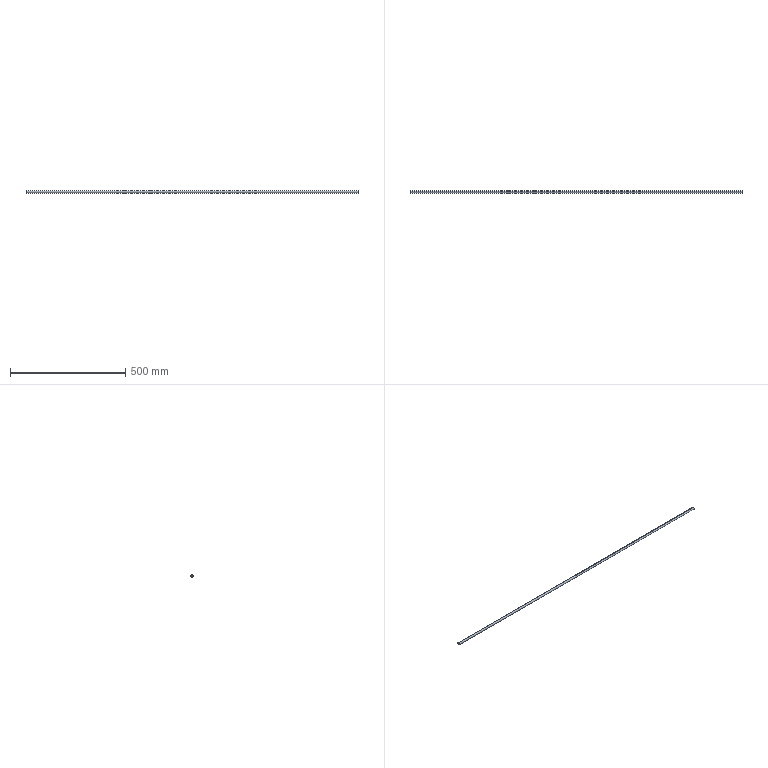Part | SolidWorks | features Revolution 1 | 1 solid | 4 faces | box 1440 x 10 x 10 mm | volume 113097 mm3 | cylinder 2 | plane 2 | commonest cylinder face diameters 10 x2
STEP:
#1=CARTESIAN_POINT('',(0.,45.,-5.));
#2=VERTEX_POINT('',#1);
#3=CARTESIAN_POINT('',(0.,45.,5.));
#4=VERTEX_POINT('',#3);
#5=CARTESIAN_POINT('',(0.,45.,0.));
#6=DIRECTION('',(1.,0.,0.));
#7=DIRECTION('',(0.,0.,-1.));
#8=AXIS2_PLACEMENT_3D('',#5,#6,#7);
#9=CIRCLE('',#8,5.);
#10=EDGE_CURVE('',#2,#4,#9,.T.);
#11=ORIENTED_EDGE('',*,*,#10,.T.);
#12=CARTESIAN_POINT('',(1440.,45.,5.));
#13=VERTEX_POINT('',#12);
#14=CARTESIAN_POINT('',(0.,45.,5.));
#15=DIRECTION('',(1.,0.,0.));
#16=VECTOR('',#15,1000.);
#17=LINE('',#14,#16);
#18=EDGE_CURVE('',#4,#13,#17,.T.);
#19=ORIENTED_EDGE('',*,*,#18,.T.);
#20=CARTESIAN_POINT('',(1440.,45.,-5.));
#21=VERTEX_POINT('',#20);
#22=CARTESIAN_POINT('',(1440.,45.,0.));
#23=DIRECTION('',(1.,0.,0.));
#24=DIRECTION('',(0.,0.,-1.));
#25=AXIS2_PLACEMENT_3D('',#22,#23,#24);
#26=CIRCLE('',#25,5.);
#27=EDGE_CURVE('',#21,#13,#26,.T.);
#28=ORIENTED_EDGE('',*,*,#27,.F.);
#29=CARTESIAN_POINT('',(0.,45.,-5.));
#30=DIRECTION('',(1.,0.,0.));
#31=VECTOR('',#30,1000.);
#32=LINE('',#29,#31);
#33=EDGE_CURVE('',#2,#21,#32,.T.);
#34=ORIENTED_EDGE('',*,*,#33,.F.);
#35=EDGE_LOOP('',(#11,#19,#28,#34));
#36=FACE_OUTER_BOUND('',#35,.T.);
#37=CARTESIAN_POINT('',(0.,45.,0.));
#38=DIRECTION('',(1.,0.,0.));
#39=DIRECTION('',(0.,0.,-1.));
#40=AXIS2_PLACEMENT_3D('',#37,#38,#39);
#41=CYLINDRICAL_SURFACE('',#40,5.);
#42=ADVANCED_FACE('',(#36),#41,.T.);
#43=ORIENTED_EDGE('',*,*,#18,.F.);
#44=CARTESIAN_POINT('',(0.,45.,0.));
#45=DIRECTION('',(1.,0.,0.));
#46=DIRECTION('',(0.,0.,-1.));
#47=AXIS2_PLACEMENT_3D('',#44,#45,#46);
#48=CIRCLE('',#47,5.);
#49=EDGE_CURVE('',#4,#2,#48,.T.);
#50=ORIENTED_EDGE('',*,*,#49,.T.);
#51=ORIENTED_EDGE('',*,*,#33,.T.);
#52=CARTESIAN_POINT('',(1440.,45.,0.));
#53=DIRECTION('',(1.,0.,0.));
#54=DIRECTION('',(0.,0.,-1.));
#55=AXIS2_PLACEMENT_3D('',#52,#53,#54);
#56=CIRCLE('',#55,5.);
#57=EDGE_CURVE('',#13,#21,#56,.T.);
#58=ORIENTED_EDGE('',*,*,#57,.F.);
#59=EDGE_LOOP('',(#43,#50,#51,#58));
#60=FACE_OUTER_BOUND('',#59,.T.);
#61=CARTESIAN_POINT('',(0.,45.,0.));
#62=DIRECTION('',(1.,0.,0.));
#63=DIRECTION('',(0.,0.,-1.));
#64=AXIS2_PLACEMENT_3D('',#61,#62,#63);
#65=CYLINDRICAL_SURFACE('',#64,5.);
#66=ADVANCED_FACE('',(#60),#65,.T.);
#67=ORIENTED_EDGE('',*,*,#10,.F.);
#68=ORIENTED_EDGE('',*,*,#49,.F.);
#69=EDGE_LOOP('',(#67,#68));
#70=FACE_OUTER_BOUND('',#69,.T.);
#71=CARTESIAN_POINT('',(0.,50.,0.));
#72=DIRECTION('',(-1.,0.,0.));
#73=DIRECTION('',(0.,0.,1.));
#74=AXIS2_PLACEMENT_3D('',#71,#72,#73);
#75=PLANE('',#74);
#76=ADVANCED_FACE('',(#70),#75,.T.);
#77=ORIENTED_EDGE('',*,*,#27,.T.);
#78=ORIENTED_EDGE('',*,*,#57,.T.);
#79=EDGE_LOOP('',(#77,#78));
#80=FACE_OUTER_BOUND('',#79,.T.);
#81=CARTESIAN_POINT('',(1440.,45.,0.));
#82=DIRECTION('',(1.,0.,0.));
#83=DIRECTION('',(0.,0.,-1.));
#84=AXIS2_PLACEMENT_3D('',#81,#82,#83);
#85=PLANE('',#84);
#86=ADVANCED_FACE('',(#80),#85,.T.);
#87=CLOSED_SHELL('',(#42,#66,#76,#86));
#88=MANIFOLD_SOLID_BREP('',#87);
#89=CARTESIAN_POINT('',(0.,0.,0.));
#90=DIRECTION('',(0.,0.,1.));
#91=DIRECTION('',(1.,0.,0.));
#92=AXIS2_PLACEMENT_3D('',#89,#90,#91);
#93=(LENGTH_UNIT()NAMED_UNIT(*)SI_UNIT(.MILLI.,.METRE.));
#94=UNCERTAINTY_MEASURE_WITH_UNIT(LENGTH_MEASURE(0.00001),#93,'','');
#95=(NAMED_UNIT(*)PLANE_ANGLE_UNIT()SI_UNIT($,.RADIAN.));
#96=(NAMED_UNIT(*)SI_UNIT($,.STERADIAN.)SOLID_ANGLE_UNIT());
#97=(GEOMETRIC_REPRESENTATION_CONTEXT(3)GLOBAL_UNCERTAINTY_ASSIGNED_CONTEXT((#94))GLOBAL_UNIT_ASSIGNED_CONTEXT((#93,#95,#96))REPRESENTATION_CONTEXT('',''));
#98=ADVANCED_BREP_SHAPE_REPRESENTATION('',(#88,#92),#97);